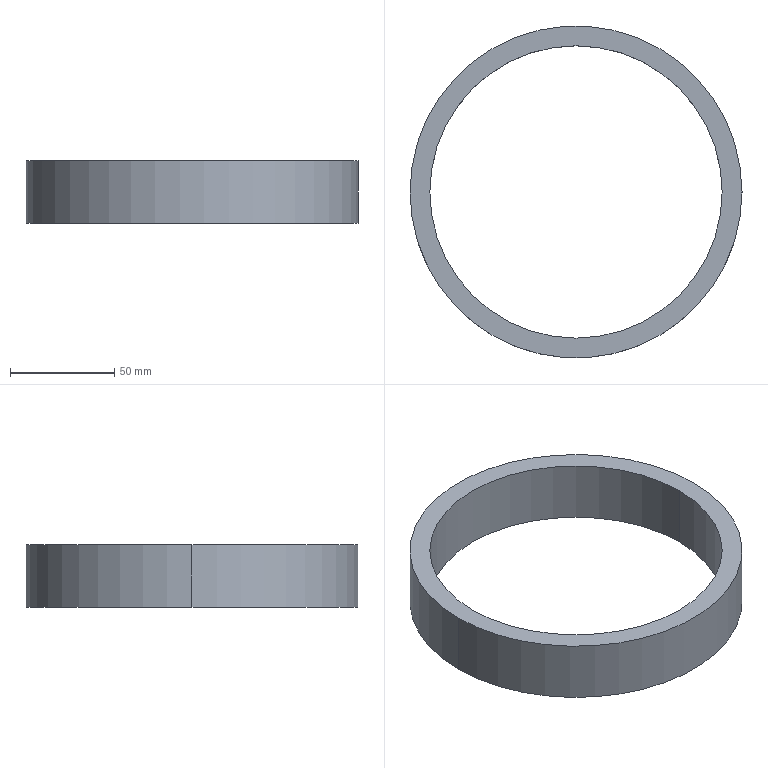Part | NX | features BREP 1 | 1 solid | 6 faces | box 159 x 159 x 30 mm | volume 133855 mm3 | cylinder 4 | plane 2 | commonest cylinder face diameters 140 x2 159 x2
STEP:
#1=CARTESIAN_POINT('',(-70.,0.,30.));
#2=VERTEX_POINT('',#1);
#3=CARTESIAN_POINT('',(70.,0.,30.));
#4=VERTEX_POINT('',#3);
#5=CARTESIAN_POINT('',(0.,0.,30.));
#6=DIRECTION('',(0.,0.,1.));
#7=DIRECTION('',(1.,0.,0.));
#8=AXIS2_PLACEMENT_3D('',#5,#6,#7);
#9=CIRCLE('',#8,70.);
#10=EDGE_CURVE('',#2,#4,#9,.T.);
#11=ORIENTED_EDGE('',*,*,#10,.T.);
#12=CARTESIAN_POINT('',(70.,0.,0.));
#13=VERTEX_POINT('',#12);
#14=CARTESIAN_POINT('',(70.,0.,30.));
#15=DIRECTION('',(0.,0.,-1.));
#16=VECTOR('',#15,1000.);
#17=LINE('',#14,#16);
#18=EDGE_CURVE('',#13,#4,#17,.F.);
#19=ORIENTED_EDGE('',*,*,#18,.F.);
#20=CARTESIAN_POINT('',(-70.,0.,0.));
#21=VERTEX_POINT('',#20);
#22=CARTESIAN_POINT('',(0.,0.,0.));
#23=DIRECTION('',(0.,0.,1.));
#24=DIRECTION('',(1.,0.,0.));
#25=AXIS2_PLACEMENT_3D('',#22,#23,#24);
#26=CIRCLE('',#25,70.);
#27=EDGE_CURVE('',#21,#13,#26,.T.);
#28=ORIENTED_EDGE('',*,*,#27,.F.);
#29=CARTESIAN_POINT('',(-70.,0.,30.));
#30=DIRECTION('',(0.,0.,-1.));
#31=VECTOR('',#30,1000.);
#32=LINE('',#29,#31);
#33=EDGE_CURVE('',#21,#2,#32,.F.);
#34=ORIENTED_EDGE('',*,*,#33,.T.);
#35=EDGE_LOOP('',(#11,#19,#28,#34));
#36=FACE_BOUND('',#35,.T.);
#37=CARTESIAN_POINT('',(0.,0.,30.));
#38=DIRECTION('',(0.,0.,-1.));
#39=DIRECTION('',(1.,0.,0.));
#40=AXIS2_PLACEMENT_3D('',#37,#38,#39);
#41=CYLINDRICAL_SURFACE('',#40,70.);
#42=ADVANCED_FACE('',(#36),#41,.F.);
#43=CARTESIAN_POINT('',(79.5,0.,30.));
#44=VERTEX_POINT('',#43);
#45=CARTESIAN_POINT('',(-79.5,0.,30.));
#46=VERTEX_POINT('',#45);
#47=CARTESIAN_POINT('',(0.,0.,30.));
#48=DIRECTION('',(0.,0.,1.));
#49=DIRECTION('',(1.,0.,0.));
#50=AXIS2_PLACEMENT_3D('',#47,#48,#49);
#51=CIRCLE('',#50,79.5);
#52=EDGE_CURVE('',#44,#46,#51,.T.);
#53=ORIENTED_EDGE('',*,*,#52,.F.);
#54=CARTESIAN_POINT('',(79.5,0.,0.));
#55=VERTEX_POINT('',#54);
#56=CARTESIAN_POINT('',(79.5,0.,30.));
#57=DIRECTION('',(0.,0.,-1.));
#58=VECTOR('',#57,1000.);
#59=LINE('',#56,#58);
#60=EDGE_CURVE('',#55,#44,#59,.F.);
#61=ORIENTED_EDGE('',*,*,#60,.F.);
#62=CARTESIAN_POINT('',(-79.5,0.,0.));
#63=VERTEX_POINT('',#62);
#64=CARTESIAN_POINT('',(0.,0.,0.));
#65=DIRECTION('',(0.,0.,1.));
#66=DIRECTION('',(1.,0.,0.));
#67=AXIS2_PLACEMENT_3D('',#64,#65,#66);
#68=CIRCLE('',#67,79.5);
#69=EDGE_CURVE('',#55,#63,#68,.T.);
#70=ORIENTED_EDGE('',*,*,#69,.T.);
#71=CARTESIAN_POINT('',(-79.5,0.,30.));
#72=DIRECTION('',(0.,0.,-1.));
#73=VECTOR('',#72,1000.);
#74=LINE('',#71,#73);
#75=EDGE_CURVE('',#63,#46,#74,.F.);
#76=ORIENTED_EDGE('',*,*,#75,.T.);
#77=EDGE_LOOP('',(#53,#61,#70,#76));
#78=FACE_BOUND('',#77,.T.);
#79=CARTESIAN_POINT('',(0.,0.,30.));
#80=DIRECTION('',(0.,0.,-1.));
#81=DIRECTION('',(1.,0.,0.));
#82=AXIS2_PLACEMENT_3D('',#79,#80,#81);
#83=CYLINDRICAL_SURFACE('',#82,79.5);
#84=ADVANCED_FACE('',(#78),#83,.T.);
#85=CARTESIAN_POINT('',(0.,0.,30.));
#86=DIRECTION('',(0.,0.,1.));
#87=DIRECTION('',(1.,0.,0.));
#88=AXIS2_PLACEMENT_3D('',#85,#86,#87);
#89=CIRCLE('',#88,79.5);
#90=EDGE_CURVE('',#46,#44,#89,.T.);
#91=ORIENTED_EDGE('',*,*,#90,.T.);
#92=ORIENTED_EDGE('',*,*,#52,.T.);
#93=EDGE_LOOP('',(#91,#92));
#94=FACE_BOUND('',#93,.T.);
#95=ORIENTED_EDGE('',*,*,#10,.F.);
#96=CARTESIAN_POINT('',(0.,0.,30.));
#97=DIRECTION('',(0.,0.,1.));
#98=DIRECTION('',(1.,0.,0.));
#99=AXIS2_PLACEMENT_3D('',#96,#97,#98);
#100=CIRCLE('',#99,70.);
#101=EDGE_CURVE('',#4,#2,#100,.T.);
#102=ORIENTED_EDGE('',*,*,#101,.F.);
#103=EDGE_LOOP('',(#95,#102));
#104=FACE_BOUND('',#103,.T.);
#105=CARTESIAN_POINT('',(0.,0.,30.));
#106=DIRECTION('',(0.,0.,1.));
#107=DIRECTION('',(-1.,0.,0.));
#108=AXIS2_PLACEMENT_3D('',#105,#106,#107);
#109=PLANE('',#108);
#110=ADVANCED_FACE('',(#94,#104),#109,.T.);
#111=CARTESIAN_POINT('',(0.,0.,0.));
#112=DIRECTION('',(0.,0.,1.));
#113=DIRECTION('',(1.,0.,0.));
#114=AXIS2_PLACEMENT_3D('',#111,#112,#113);
#115=CIRCLE('',#114,79.5);
#116=EDGE_CURVE('',#63,#55,#115,.T.);
#117=ORIENTED_EDGE('',*,*,#116,.F.);
#118=ORIENTED_EDGE('',*,*,#69,.F.);
#119=EDGE_LOOP('',(#117,#118));
#120=FACE_BOUND('',#119,.T.);
#121=ORIENTED_EDGE('',*,*,#27,.T.);
#122=CARTESIAN_POINT('',(0.,0.,0.));
#123=DIRECTION('',(0.,0.,1.));
#124=DIRECTION('',(1.,0.,0.));
#125=AXIS2_PLACEMENT_3D('',#122,#123,#124);
#126=CIRCLE('',#125,70.);
#127=EDGE_CURVE('',#13,#21,#126,.T.);
#128=ORIENTED_EDGE('',*,*,#127,.T.);
#129=EDGE_LOOP('',(#121,#128));
#130=FACE_BOUND('',#129,.T.);
#131=CARTESIAN_POINT('',(0.,0.,0.));
#132=DIRECTION('',(0.,0.,1.));
#133=DIRECTION('',(-1.,0.,0.));
#134=AXIS2_PLACEMENT_3D('',#131,#132,#133);
#135=PLANE('',#134);
#136=ADVANCED_FACE('',(#120,#130),#135,.F.);
#137=ORIENTED_EDGE('',*,*,#60,.T.);
#138=ORIENTED_EDGE('',*,*,#90,.F.);
#139=ORIENTED_EDGE('',*,*,#75,.F.);
#140=ORIENTED_EDGE('',*,*,#116,.T.);
#141=EDGE_LOOP('',(#137,#138,#139,#140));
#142=FACE_BOUND('',#141,.T.);
#143=CARTESIAN_POINT('',(0.,0.,30.));
#144=DIRECTION('',(0.,0.,-1.));
#145=DIRECTION('',(1.,0.,0.));
#146=AXIS2_PLACEMENT_3D('',#143,#144,#145);
#147=CYLINDRICAL_SURFACE('',#146,79.5);
#148=ADVANCED_FACE('',(#142),#147,.T.);
#149=ORIENTED_EDGE('',*,*,#18,.T.);
#150=ORIENTED_EDGE('',*,*,#101,.T.);
#151=ORIENTED_EDGE('',*,*,#33,.F.);
#152=ORIENTED_EDGE('',*,*,#127,.F.);
#153=EDGE_LOOP('',(#149,#150,#151,#152));
#154=FACE_BOUND('',#153,.T.);
#155=CARTESIAN_POINT('',(0.,0.,30.));
#156=DIRECTION('',(0.,0.,-1.));
#157=DIRECTION('',(1.,0.,0.));
#158=AXIS2_PLACEMENT_3D('',#155,#156,#157);
#159=CYLINDRICAL_SURFACE('',#158,70.);
#160=ADVANCED_FACE('',(#154),#159,.F.);
#161=CLOSED_SHELL('',(#42,#84,#110,#136,#148,#160));
#162=MANIFOLD_SOLID_BREP('',#161);
#163=(LENGTH_UNIT()NAMED_UNIT(*)SI_UNIT(.MILLI.,.METRE.));
#164=UNCERTAINTY_MEASURE_WITH_UNIT(LENGTH_MEASURE(0.00001),#163,'','');
#165=(NAMED_UNIT(*)PLANE_ANGLE_UNIT()SI_UNIT($,.RADIAN.));
#166=(NAMED_UNIT(*)SI_UNIT($,.STERADIAN.)SOLID_ANGLE_UNIT());
#167=(GEOMETRIC_REPRESENTATION_CONTEXT(3)GLOBAL_UNCERTAINTY_ASSIGNED_CONTEXT((#164))GLOBAL_UNIT_ASSIGNED_CONTEXT((#163,#165,#166))REPRESENTATION_CONTEXT('',''));
#168=ADVANCED_BREP_SHAPE_REPRESENTATION('',(#162),#167);